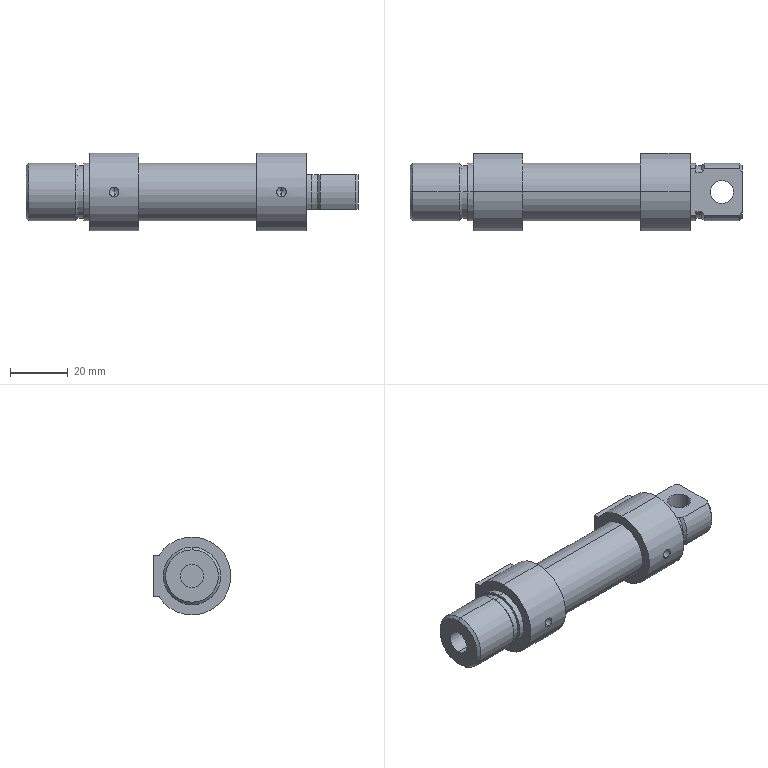Part | STEP file | 4935_DGS_16_1_P_z_HI | 1 solid | 71 faces | box 115 x 27 x 27 mm | volume 36319 mm3 | cylinder 34 | plane 21 | cone 16 | commonest cylinder face diameters 20 x10 27 x6 3.3 x4 8 x4 8.566 x4 18.159 x4